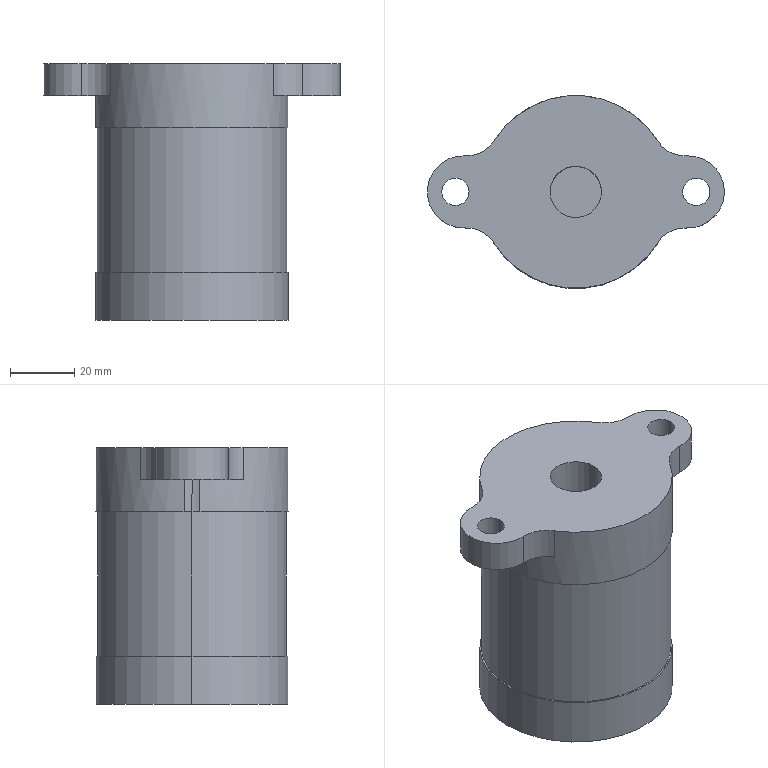Part | SolidWorks | features ICE 5, Cut 2, Extrusion 1, Fillet 1 | 1 solid | 33 faces | box 92.5 x 60 x 80 mm | volume 214232 mm3 | cylinder 23 | plane 10 | commonest cylinder face diameters 16 x6 8.5 x4 20 x4 60 x4 22.5 x3 59 x2
STEP:
#1=CARTESIAN_POINT('',(45.5,0.,-9.));
#2=VERTEX_POINT('',#1);
#3=CARTESIAN_POINT('',(29.5,0.,-9.));
#4=VERTEX_POINT('',#3);
#5=CARTESIAN_POINT('',(37.5,0.,-9.));
#6=DIRECTION('',(0.,0.,-1.));
#7=DIRECTION('',(-1.,0.,0.));
#8=AXIS2_PLACEMENT_3D('',#5,#6,#7);
#9=CIRCLE('',#8,8.);
#10=EDGE_CURVE('',#2,#4,#9,.T.);
#11=ORIENTED_EDGE('',*,*,#10,.F.);
#12=CARTESIAN_POINT('',(45.5,0.,-10.));
#13=VERTEX_POINT('',#12);
#14=CARTESIAN_POINT('',(45.5,0.,-9.));
#15=DIRECTION('',(0.,0.,-1.));
#16=VECTOR('',#15,1000.);
#17=LINE('',#14,#16);
#18=EDGE_CURVE('',#2,#13,#17,.T.);
#19=ORIENTED_EDGE('',*,*,#18,.T.);
#20=CARTESIAN_POINT('',(29.897,-2.488,-10.));
#21=VERTEX_POINT('',#20);
#22=CARTESIAN_POINT('',(37.5,0.,-10.));
#23=DIRECTION('',(0.,0.,-1.));
#24=DIRECTION('',(-1.,0.,0.));
#25=AXIS2_PLACEMENT_3D('',#22,#23,#24);
#26=CIRCLE('',#25,8.);
#27=EDGE_CURVE('',#13,#21,#26,.T.);
#28=ORIENTED_EDGE('',*,*,#27,.T.);
#29=CARTESIAN_POINT('',(29.897,-2.488,-20.));
#30=VERTEX_POINT('',#29);
#31=CARTESIAN_POINT('',(29.897,-2.488,-10.));
#32=DIRECTION('',(0.,0.,-1.));
#33=VECTOR('',#32,1000.);
#34=LINE('',#31,#33);
#35=EDGE_CURVE('',#21,#30,#34,.T.);
#36=ORIENTED_EDGE('',*,*,#35,.T.);
#37=CARTESIAN_POINT('',(29.5,0.,-20.));
#38=VERTEX_POINT('',#37);
#39=CARTESIAN_POINT('',(37.5,0.,-20.));
#40=DIRECTION('',(0.,0.,1.));
#41=DIRECTION('',(1.,0.,0.));
#42=AXIS2_PLACEMENT_3D('',#39,#40,#41);
#43=CIRCLE('',#42,8.);
#44=EDGE_CURVE('',#38,#30,#43,.T.);
#45=ORIENTED_EDGE('',*,*,#44,.F.);
#46=CARTESIAN_POINT('',(29.5,0.,-9.));
#47=DIRECTION('',(0.,0.,-1.));
#48=VECTOR('',#47,1000.);
#49=LINE('',#46,#48);
#50=EDGE_CURVE('',#4,#38,#49,.T.);
#51=ORIENTED_EDGE('',*,*,#50,.F.);
#52=EDGE_LOOP('',(#11,#19,#28,#36,#45,#51));
#53=FACE_OUTER_BOUND('',#52,.T.);
#54=CARTESIAN_POINT('',(37.5,0.,-9.));
#55=DIRECTION('',(0.,0.,-1.));
#56=DIRECTION('',(-1.,0.,0.));
#57=AXIS2_PLACEMENT_3D('',#54,#55,#56);
#58=CYLINDRICAL_SURFACE('',#57,8.);
#59=ADVANCED_FACE('',(#53),#58,.F.);
#60=CARTESIAN_POINT('',(-29.5,0.,-9.));
#61=VERTEX_POINT('',#60);
#62=CARTESIAN_POINT('',(-45.5,0.,-9.));
#63=VERTEX_POINT('',#62);
#64=CARTESIAN_POINT('',(-37.5,0.,-9.));
#65=DIRECTION('',(0.,0.,-1.));
#66=DIRECTION('',(-1.,0.,0.));
#67=AXIS2_PLACEMENT_3D('',#64,#65,#66);
#68=CIRCLE('',#67,8.);
#69=EDGE_CURVE('',#61,#63,#68,.T.);
#70=ORIENTED_EDGE('',*,*,#69,.F.);
#71=CARTESIAN_POINT('',(-29.5,0.,-20.));
#72=VERTEX_POINT('',#71);
#73=CARTESIAN_POINT('',(-29.5,0.,-9.));
#74=DIRECTION('',(0.,0.,-1.));
#75=VECTOR('',#74,1000.);
#76=LINE('',#73,#75);
#77=EDGE_CURVE('',#61,#72,#76,.T.);
#78=ORIENTED_EDGE('',*,*,#77,.T.);
#79=CARTESIAN_POINT('',(-29.897,-2.488,-20.));
#80=VERTEX_POINT('',#79);
#81=CARTESIAN_POINT('',(-37.5,0.,-20.));
#82=DIRECTION('',(0.,0.,1.));
#83=DIRECTION('',(1.,0.,0.));
#84=AXIS2_PLACEMENT_3D('',#81,#82,#83);
#85=CIRCLE('',#84,8.);
#86=EDGE_CURVE('',#80,#72,#85,.T.);
#87=ORIENTED_EDGE('',*,*,#86,.F.);
#88=CARTESIAN_POINT('',(-29.897,-2.488,-10.));
#89=VERTEX_POINT('',#88);
#90=CARTESIAN_POINT('',(-29.897,-2.488,-10.));
#91=DIRECTION('',(0.,0.,1.));
#92=VECTOR('',#91,1000.);
#93=LINE('',#90,#92);
#94=EDGE_CURVE('',#80,#89,#93,.T.);
#95=ORIENTED_EDGE('',*,*,#94,.T.);
#96=CARTESIAN_POINT('',(-45.5,0.,-10.));
#97=VERTEX_POINT('',#96);
#98=CARTESIAN_POINT('',(-37.5,0.,-10.));
#99=DIRECTION('',(0.,0.,-1.));
#100=DIRECTION('',(-1.,0.,0.));
#101=AXIS2_PLACEMENT_3D('',#98,#99,#100);
#102=CIRCLE('',#101,8.);
#103=EDGE_CURVE('',#89,#97,#102,.T.);
#104=ORIENTED_EDGE('',*,*,#103,.T.);
#105=CARTESIAN_POINT('',(-45.5,0.,-9.));
#106=DIRECTION('',(0.,0.,-1.));
#107=VECTOR('',#106,1000.);
#108=LINE('',#105,#107);
#109=EDGE_CURVE('',#63,#97,#108,.T.);
#110=ORIENTED_EDGE('',*,*,#109,.F.);
#111=EDGE_LOOP('',(#70,#78,#87,#95,#104,#110));
#112=FACE_OUTER_BOUND('',#111,.T.);
#113=CARTESIAN_POINT('',(-37.5,0.,-9.));
#114=DIRECTION('',(0.,0.,-1.));
#115=DIRECTION('',(-1.,0.,0.));
#116=AXIS2_PLACEMENT_3D('',#113,#114,#115);
#117=CYLINDRICAL_SURFACE('',#116,8.);
#118=ADVANCED_FACE('',(#112),#117,.F.);
#119=CARTESIAN_POINT('',(34.421,-11.235,-10.));
#120=VERTEX_POINT('',#119);
#121=CARTESIAN_POINT('',(46.25,0.,-10.));
#122=VERTEX_POINT('',#121);
#123=CARTESIAN_POINT('',(35.,0.,-10.));
#124=DIRECTION('',(0.,0.,1.));
#125=DIRECTION('',(1.,0.,0.));
#126=AXIS2_PLACEMENT_3D('',#123,#124,#125);
#127=CIRCLE('',#126,11.25);
#128=EDGE_CURVE('',#120,#122,#127,.T.);
#129=ORIENTED_EDGE('',*,*,#128,.T.);
#130=CARTESIAN_POINT('',(46.25,0.,0.));
#131=VERTEX_POINT('',#130);
#132=CARTESIAN_POINT('',(46.25,0.,-10.));
#133=DIRECTION('',(0.,0.,1.));
#134=VECTOR('',#133,1000.);
#135=LINE('',#132,#134);
#136=EDGE_CURVE('',#122,#131,#135,.T.);
#137=ORIENTED_EDGE('',*,*,#136,.T.);
#138=CARTESIAN_POINT('',(34.421,-11.235,0.));
#139=VERTEX_POINT('',#138);
#140=CARTESIAN_POINT('',(35.,0.,0.));
#141=DIRECTION('',(0.,0.,1.));
#142=DIRECTION('',(1.,0.,0.));
#143=AXIS2_PLACEMENT_3D('',#140,#141,#142);
#144=CIRCLE('',#143,11.25);
#145=EDGE_CURVE('',#139,#131,#144,.T.);
#146=ORIENTED_EDGE('',*,*,#145,.F.);
#147=CARTESIAN_POINT('',(34.421,-11.235,-10.));
#148=DIRECTION('',(0.,0.,-1.));
#149=VECTOR('',#148,1000.);
#150=LINE('',#147,#149);
#151=EDGE_CURVE('',#139,#120,#150,.T.);
#152=ORIENTED_EDGE('',*,*,#151,.T.);
#153=EDGE_LOOP('',(#129,#137,#146,#152));
#154=FACE_OUTER_BOUND('',#153,.T.);
#155=CARTESIAN_POINT('',(35.,0.,-10.));
#156=DIRECTION('',(0.,0.,1.));
#157=DIRECTION('',(1.,0.,0.));
#158=AXIS2_PLACEMENT_3D('',#155,#156,#157);
#159=CYLINDRICAL_SURFACE('',#158,11.25);
#160=ADVANCED_FACE('',(#154),#159,.T.);
#161=CARTESIAN_POINT('',(-8.,0.,-65.));
#162=VERTEX_POINT('',#161);
#163=CARTESIAN_POINT('',(8.,0.,-65.));
#164=VERTEX_POINT('',#163);
#165=CARTESIAN_POINT('',(0.,0.,-65.));
#166=DIRECTION('',(0.,0.,1.));
#167=DIRECTION('',(1.,0.,0.));
#168=AXIS2_PLACEMENT_3D('',#165,#166,#167);
#169=CIRCLE('',#168,8.);
#170=EDGE_CURVE('',#162,#164,#169,.T.);
#171=ORIENTED_EDGE('',*,*,#170,.F.);
#172=CARTESIAN_POINT('',(-8.,0.,0.));
#173=VERTEX_POINT('',#172);
#174=CARTESIAN_POINT('',(-8.,0.,-65.));
#175=DIRECTION('',(0.,0.,1.));
#176=VECTOR('',#175,1000.);
#177=LINE('',#174,#176);
#178=EDGE_CURVE('',#162,#173,#177,.T.);
#179=ORIENTED_EDGE('',*,*,#178,.T.);
#180=CARTESIAN_POINT('',(8.,0.,0.));
#181=VERTEX_POINT('',#180);
#182=CARTESIAN_POINT('',(0.,0.,0.));
#183=DIRECTION('',(0.,0.,1.));
#184=DIRECTION('',(1.,0.,0.));
#185=AXIS2_PLACEMENT_3D('',#182,#183,#184);
#186=CIRCLE('',#185,8.);
#187=EDGE_CURVE('',#173,#181,#186,.T.);
#188=ORIENTED_EDGE('',*,*,#187,.T.);
#189=CARTESIAN_POINT('',(8.,0.,-65.));
#190=DIRECTION('',(0.,0.,1.));
#191=VECTOR('',#190,1000.);
#192=LINE('',#189,#191);
#193=EDGE_CURVE('',#164,#181,#192,.T.);
#194=ORIENTED_EDGE('',*,*,#193,.F.);
#195=EDGE_LOOP('',(#171,#179,#188,#194));
#196=FACE_OUTER_BOUND('',#195,.T.);
#197=CARTESIAN_POINT('',(0.,0.,-65.));
#198=DIRECTION('',(0.,0.,1.));
#199=DIRECTION('',(1.,0.,0.));
#200=AXIS2_PLACEMENT_3D('',#197,#198,#199);
#201=CYLINDRICAL_SURFACE('',#200,8.);
#202=ADVANCED_FACE('',(#196),#201,.F.);
#203=CARTESIAN_POINT('',(-30.,0.,-80.));
#204=VERTEX_POINT('',#203);
#205=CARTESIAN_POINT('',(30.,0.,-80.));
#206=VERTEX_POINT('',#205);
#207=CARTESIAN_POINT('',(0.,0.,-80.));
#208=DIRECTION('',(0.,0.,-1.));
#209=DIRECTION('',(-1.,0.,0.));
#210=AXIS2_PLACEMENT_3D('',#207,#208,#209);
#211=CIRCLE('',#210,30.);
#212=EDGE_CURVE('',#204,#206,#211,.T.);
#213=ORIENTED_EDGE('',*,*,#212,.F.);
#214=CARTESIAN_POINT('',(-30.,0.,-65.));
#215=VERTEX_POINT('',#214);
#216=CARTESIAN_POINT('',(-30.,0.,-80.));
#217=DIRECTION('',(0.,0.,1.));
#218=VECTOR('',#217,1000.);
#219=LINE('',#216,#218);
#220=EDGE_CURVE('',#204,#215,#219,.T.);
#221=ORIENTED_EDGE('',*,*,#220,.T.);
#222=CARTESIAN_POINT('',(30.,0.,-65.));
#223=VERTEX_POINT('',#222);
#224=CARTESIAN_POINT('',(0.,0.,-65.));
#225=DIRECTION('',(0.,0.,-1.));
#226=DIRECTION('',(-1.,0.,0.));
#227=AXIS2_PLACEMENT_3D('',#224,#225,#226);
#228=CIRCLE('',#227,30.);
#229=EDGE_CURVE('',#215,#223,#228,.T.);
#230=ORIENTED_EDGE('',*,*,#229,.T.);
#231=CARTESIAN_POINT('',(30.,0.,-80.));
#232=DIRECTION('',(0.,0.,1.));
#233=VECTOR('',#232,1000.);
#234=LINE('',#231,#233);
#235=EDGE_CURVE('',#206,#223,#234,.T.);
#236=ORIENTED_EDGE('',*,*,#235,.F.);
#237=EDGE_LOOP('',(#213,#221,#230,#236));
#238=FACE_OUTER_BOUND('',#237,.T.);
#239=CARTESIAN_POINT('',(0.,0.,-80.));
#240=DIRECTION('',(0.,0.,1.));
#241=DIRECTION('',(1.,0.,0.));
#242=AXIS2_PLACEMENT_3D('',#239,#240,#241);
#243=CYLINDRICAL_SURFACE('',#242,30.);
#244=ADVANCED_FACE('',(#238),#243,.T.);
#245=CARTESIAN_POINT('',(-29.5,0.,-65.));
#246=VERTEX_POINT('',#245);
#247=CARTESIAN_POINT('',(29.5,0.,-65.));
#248=VERTEX_POINT('',#247);
#249=CARTESIAN_POINT('',(0.,0.,-65.));
#250=DIRECTION('',(0.,0.,-1.));
#251=DIRECTION('',(-1.,0.,0.));
#252=AXIS2_PLACEMENT_3D('',#249,#250,#251);
#253=CIRCLE('',#252,29.5);
#254=EDGE_CURVE('',#246,#248,#253,.T.);
#255=ORIENTED_EDGE('',*,*,#254,.F.);
#256=CARTESIAN_POINT('',(-29.5,0.,-65.));
#257=DIRECTION('',(0.,0.,1.));
#258=VECTOR('',#257,1000.);
#259=LINE('',#256,#258);
#260=EDGE_CURVE('',#246,#72,#259,.T.);
#261=ORIENTED_EDGE('',*,*,#260,.T.);
#262=CARTESIAN_POINT('',(0.,0.,-20.));
#263=DIRECTION('',(0.,0.,-1.));
#264=DIRECTION('',(1.,0.,0.));
#265=AXIS2_PLACEMENT_3D('',#262,#263,#264);
#266=CIRCLE('',#265,29.5);
#267=EDGE_CURVE('',#72,#38,#266,.T.);
#268=ORIENTED_EDGE('',*,*,#267,.T.);
#269=CARTESIAN_POINT('',(29.5,0.,-65.));
#270=DIRECTION('',(0.,0.,1.));
#271=VECTOR('',#270,1000.);
#272=LINE('',#269,#271);
#273=EDGE_CURVE('',#248,#38,#272,.T.);
#274=ORIENTED_EDGE('',*,*,#273,.F.);
#275=EDGE_LOOP('',(#255,#261,#268,#274));
#276=FACE_OUTER_BOUND('',#275,.T.);
#277=CARTESIAN_POINT('',(0.,0.,-65.));
#278=DIRECTION('',(0.,0.,1.));
#279=DIRECTION('',(1.,0.,0.));
#280=AXIS2_PLACEMENT_3D('',#277,#278,#279);
#281=CYLINDRICAL_SURFACE('',#280,29.5);
#282=ADVANCED_FACE('',(#276),#281,.T.);
#283=CARTESIAN_POINT('',(-33.25,0.,0.));
#284=VERTEX_POINT('',#283);
#285=CARTESIAN_POINT('',(-41.75,0.,0.));
#286=VERTEX_POINT('',#285);
#287=CARTESIAN_POINT('',(-37.5,0.,0.));
#288=DIRECTION('',(0.,0.,-1.));
#289=DIRECTION('',(-1.,0.,0.));
#290=AXIS2_PLACEMENT_3D('',#287,#288,#289);
#291=CIRCLE('',#290,4.25);
#292=EDGE_CURVE('',#284,#286,#291,.T.);
#293=ORIENTED_EDGE('',*,*,#292,.F.);
#294=CARTESIAN_POINT('',(-33.25,0.,-9.));
#295=VERTEX_POINT('',#294);
#296=CARTESIAN_POINT('',(-33.25,0.,0.));
#297=DIRECTION('',(0.,0.,-1.));
#298=VECTOR('',#297,1000.);
#299=LINE('',#296,#298);
#300=EDGE_CURVE('',#284,#295,#299,.T.);
#301=ORIENTED_EDGE('',*,*,#300,.T.);
#302=CARTESIAN_POINT('',(-41.75,0.,-9.));
#303=VERTEX_POINT('',#302);
#304=CARTESIAN_POINT('',(-37.5,0.,-9.));
#305=DIRECTION('',(0.,0.,1.));
#306=DIRECTION('',(-1.,0.,0.));
#307=AXIS2_PLACEMENT_3D('',#304,#305,#306);
#308=CIRCLE('',#307,4.25);
#309=EDGE_CURVE('',#303,#295,#308,.T.);
#310=ORIENTED_EDGE('',*,*,#309,.F.);
#311=CARTESIAN_POINT('',(-41.75,0.,0.));
#312=DIRECTION('',(0.,0.,-1.));
#313=VECTOR('',#312,1000.);
#314=LINE('',#311,#313);
#315=EDGE_CURVE('',#286,#303,#314,.T.);
#316=ORIENTED_EDGE('',*,*,#315,.F.);
#317=EDGE_LOOP('',(#293,#301,#310,#316));
#318=FACE_OUTER_BOUND('',#317,.T.);
#319=CARTESIAN_POINT('',(-37.5,0.,0.));
#320=DIRECTION('',(0.,0.,-1.));
#321=DIRECTION('',(-1.,0.,0.));
#322=AXIS2_PLACEMENT_3D('',#319,#320,#321);
#323=CYLINDRICAL_SURFACE('',#322,4.25);
#324=ADVANCED_FACE('',(#318),#323,.F.);
#325=CARTESIAN_POINT('',(41.75,0.,0.));
#326=VERTEX_POINT('',#325);
#327=CARTESIAN_POINT('',(33.25,0.,0.));
#328=VERTEX_POINT('',#327);
#329=CARTESIAN_POINT('',(37.5,0.,0.));
#330=DIRECTION('',(0.,0.,-1.));
#331=DIRECTION('',(-1.,0.,0.));
#332=AXIS2_PLACEMENT_3D('',#329,#330,#331);
#333=CIRCLE('',#332,4.25);
#334=EDGE_CURVE('',#326,#328,#333,.T.);
#335=ORIENTED_EDGE('',*,*,#334,.F.);
#336=CARTESIAN_POINT('',(41.75,0.,-9.));
#337=VERTEX_POINT('',#336);
#338=CARTESIAN_POINT('',(41.75,0.,0.));
#339=DIRECTION('',(0.,0.,-1.));
#340=VECTOR('',#339,1000.);
#341=LINE('',#338,#340);
#342=EDGE_CURVE('',#326,#337,#341,.T.);
#343=ORIENTED_EDGE('',*,*,#342,.T.);
#344=CARTESIAN_POINT('',(33.25,0.,-9.));
#345=VERTEX_POINT('',#344);
#346=CARTESIAN_POINT('',(37.5,0.,-9.));
#347=DIRECTION('',(0.,0.,1.));
#348=DIRECTION('',(-1.,0.,0.));
#349=AXIS2_PLACEMENT_3D('',#346,#347,#348);
#350=CIRCLE('',#349,4.25);
#351=EDGE_CURVE('',#345,#337,#350,.T.);
#352=ORIENTED_EDGE('',*,*,#351,.F.);
#353=CARTESIAN_POINT('',(33.25,0.,0.));
#354=DIRECTION('',(0.,0.,-1.));
#355=VECTOR('',#354,1000.);
#356=LINE('',#353,#355);
#357=EDGE_CURVE('',#328,#345,#356,.T.);
#358=ORIENTED_EDGE('',*,*,#357,.F.);
#359=EDGE_LOOP('',(#335,#343,#352,#358));
#360=FACE_OUTER_BOUND('',#359,.T.);
#361=CARTESIAN_POINT('',(37.5,0.,0.));
#362=DIRECTION('',(0.,0.,-1.));
#363=DIRECTION('',(-1.,0.,0.));
#364=AXIS2_PLACEMENT_3D('',#361,#362,#363);
#365=CYLINDRICAL_SURFACE('',#364,4.25);
#366=ADVANCED_FACE('',(#360),#365,.F.);
#367=ORIENTED_EDGE('',*,*,#44,.T.);
#368=CARTESIAN_POINT('',(0.,0.,-20.));
#369=DIRECTION('',(0.,0.,1.));
#370=DIRECTION('',(1.,0.,0.));
#371=AXIS2_PLACEMENT_3D('',#368,#369,#370);
#372=CIRCLE('',#371,30.);
#373=EDGE_CURVE('',#80,#30,#372,.T.);
#374=ORIENTED_EDGE('',*,*,#373,.F.);
#375=ORIENTED_EDGE('',*,*,#86,.T.);
#376=CARTESIAN_POINT('',(0.,0.,-20.));
#377=DIRECTION('',(0.,0.,-1.));
#378=DIRECTION('',(1.,0.,0.));
#379=AXIS2_PLACEMENT_3D('',#376,#377,#378);
#380=CIRCLE('',#379,29.5);
#381=EDGE_CURVE('',#38,#72,#380,.T.);
#382=ORIENTED_EDGE('',*,*,#381,.F.);
#383=EDGE_LOOP('',(#367,#374,#375,#382));
#384=FACE_OUTER_BOUND('',#383,.T.);
#385=CARTESIAN_POINT('',(0.,0.,-20.));
#386=DIRECTION('',(0.,0.,1.));
#387=DIRECTION('',(1.,0.,0.));
#388=AXIS2_PLACEMENT_3D('',#385,#386,#387);
#389=PLANE('',#388);
#390=ADVANCED_FACE('',(#384),#389,.F.);
#391=CARTESIAN_POINT('',(29.897,2.488,-20.));
#392=VERTEX_POINT('',#391);
#393=CARTESIAN_POINT('',(37.5,0.,-20.));
#394=DIRECTION('',(0.,0.,1.));
#395=DIRECTION('',(1.,0.,0.));
#396=AXIS2_PLACEMENT_3D('',#393,#394,#395);
#397=CIRCLE('',#396,8.);
#398=EDGE_CURVE('',#392,#38,#397,.T.);
#399=ORIENTED_EDGE('',*,*,#398,.T.);
#400=ORIENTED_EDGE('',*,*,#267,.F.);
#401=CARTESIAN_POINT('',(-29.897,2.488,-20.));
#402=VERTEX_POINT('',#401);
#403=CARTESIAN_POINT('',(-37.5,0.,-20.));
#404=DIRECTION('',(0.,0.,1.));
#405=DIRECTION('',(1.,0.,0.));
#406=AXIS2_PLACEMENT_3D('',#403,#404,#405);
#407=CIRCLE('',#406,8.);
#408=EDGE_CURVE('',#72,#402,#407,.T.);
#409=ORIENTED_EDGE('',*,*,#408,.T.);
#410=CARTESIAN_POINT('',(0.,0.,-20.));
#411=DIRECTION('',(0.,0.,1.));
#412=DIRECTION('',(1.,0.,0.));
#413=AXIS2_PLACEMENT_3D('',#410,#411,#412);
#414=CIRCLE('',#413,30.);
#415=EDGE_CURVE('',#392,#402,#414,.T.);
#416=ORIENTED_EDGE('',*,*,#415,.F.);
#417=EDGE_LOOP('',(#399,#400,#409,#416));
#418=FACE_OUTER_BOUND('',#417,.T.);
#419=CARTESIAN_POINT('',(0.,0.,-20.));
#420=DIRECTION('',(0.,0.,1.));
#421=DIRECTION('',(1.,0.,0.));
#422=AXIS2_PLACEMENT_3D('',#419,#420,#421);
#423=PLANE('',#422);
#424=ADVANCED_FACE('',(#418),#423,.F.);
#425=CARTESIAN_POINT('',(25.43,15.916,-10.));
#426=VERTEX_POINT('',#425);
#427=CARTESIAN_POINT('',(29.897,2.488,-10.));
#428=VERTEX_POINT('',#427);
#429=CARTESIAN_POINT('',(0.,0.,-10.));
#430=DIRECTION('',(0.,0.,-1.));
#431=DIRECTION('',(1.,0.,0.));
#432=AXIS2_PLACEMENT_3D('',#429,#430,#431);
#433=CIRCLE('',#432,30.);
#434=EDGE_CURVE('',#426,#428,#433,.T.);
#435=ORIENTED_EDGE('',*,*,#434,.T.);
#436=CARTESIAN_POINT('',(29.897,2.488,-10.));
#437=DIRECTION('',(0.,0.,1.));
#438=VECTOR('',#437,1000.);
#439=LINE('',#436,#438);
#440=EDGE_CURVE('',#392,#428,#439,.T.);
#441=ORIENTED_EDGE('',*,*,#440,.F.);
#442=ORIENTED_EDGE('',*,*,#415,.T.);
#443=CARTESIAN_POINT('',(-29.897,2.488,-10.));
#444=VERTEX_POINT('',#443);
#445=CARTESIAN_POINT('',(-29.897,2.488,-10.));
#446=DIRECTION('',(0.,0.,-1.));
#447=VECTOR('',#446,1000.);
#448=LINE('',#445,#447);
#449=EDGE_CURVE('',#444,#402,#448,.T.);
#450=ORIENTED_EDGE('',*,*,#449,.F.);
#451=CARTESIAN_POINT('',(-25.43,15.916,-10.));
#452=VERTEX_POINT('',#451);
#453=CARTESIAN_POINT('',(0.,0.,-10.));
#454=DIRECTION('',(0.,0.,-1.));
#455=DIRECTION('',(1.,0.,0.));
#456=AXIS2_PLACEMENT_3D('',#453,#454,#455);
#457=CIRCLE('',#456,30.);
#458=EDGE_CURVE('',#444,#452,#457,.T.);
#459=ORIENTED_EDGE('',*,*,#458,.T.);
#460=CARTESIAN_POINT('',(-25.43,15.916,0.));
#461=VERTEX_POINT('',#460);
#462=CARTESIAN_POINT('',(-25.43,15.916,-20.));
#463=DIRECTION('',(0.,0.,1.));
#464=VECTOR('',#463,1000.);
#465=LINE('',#462,#464);
#466=EDGE_CURVE('',#452,#461,#465,.T.);
#467=ORIENTED_EDGE('',*,*,#466,.T.);
#468=CARTESIAN_POINT('',(25.43,15.916,0.));
#469=VERTEX_POINT('',#468);
#470=CARTESIAN_POINT('',(0.,0.,0.));
#471=DIRECTION('',(0.,0.,1.));
#472=DIRECTION('',(1.,0.,0.));
#473=AXIS2_PLACEMENT_3D('',#470,#471,#472);
#474=CIRCLE('',#473,30.);
#475=EDGE_CURVE('',#469,#461,#474,.T.);
#476=ORIENTED_EDGE('',*,*,#475,.F.);
#477=CARTESIAN_POINT('',(25.43,15.916,-20.));
#478=DIRECTION('',(0.,0.,-1.));
#479=VECTOR('',#478,1000.);
#480=LINE('',#477,#479);
#481=EDGE_CURVE('',#469,#426,#480,.T.);
#482=ORIENTED_EDGE('',*,*,#481,.T.);
#483=EDGE_LOOP('',(#435,#441,#442,#450,#459,#467,#476,#482));
#484=FACE_OUTER_BOUND('',#483,.T.);
#485=CARTESIAN_POINT('',(0.,0.,-20.));
#486=DIRECTION('',(0.,0.,1.));
#487=DIRECTION('',(1.,0.,0.));
#488=AXIS2_PLACEMENT_3D('',#485,#486,#487);
#489=CYLINDRICAL_SURFACE('',#488,30.);
#490=ADVANCED_FACE('',(#484),#489,.T.);
#491=ORIENTED_EDGE('',*,*,#373,.T.);
#492=ORIENTED_EDGE('',*,*,#35,.F.);
#493=CARTESIAN_POINT('',(25.43,-15.916,-10.));
#494=VERTEX_POINT('',#493);
#495=CARTESIAN_POINT('',(0.,0.,-10.));
#496=DIRECTION('',(0.,0.,-1.));
#497=DIRECTION('',(1.,0.,0.));
#498=AXIS2_PLACEMENT_3D('',#495,#496,#497);
#499=CIRCLE('',#498,30.);
#500=EDGE_CURVE('',#21,#494,#499,.T.);
#501=ORIENTED_EDGE('',*,*,#500,.T.);
#502=CARTESIAN_POINT('',(25.43,-15.916,0.));
#503=VERTEX_POINT('',#502);
#504=CARTESIAN_POINT('',(25.43,-15.916,-20.));
#505=DIRECTION('',(0.,0.,1.));
#506=VECTOR('',#505,1000.);
#507=LINE('',#504,#506);
#508=EDGE_CURVE('',#494,#503,#507,.T.);
#509=ORIENTED_EDGE('',*,*,#508,.T.);
#510=CARTESIAN_POINT('',(-25.43,-15.916,0.));
#511=VERTEX_POINT('',#510);
#512=CARTESIAN_POINT('',(0.,0.,0.));
#513=DIRECTION('',(0.,0.,1.));
#514=DIRECTION('',(1.,0.,0.));
#515=AXIS2_PLACEMENT_3D('',#512,#513,#514);
#516=CIRCLE('',#515,30.);
#517=EDGE_CURVE('',#511,#503,#516,.T.);
#518=ORIENTED_EDGE('',*,*,#517,.F.);
#519=CARTESIAN_POINT('',(-25.43,-15.916,-10.));
#520=VERTEX_POINT('',#519);
#521=CARTESIAN_POINT('',(-25.43,-15.916,-20.));
#522=DIRECTION('',(0.,0.,-1.));
#523=VECTOR('',#522,1000.);
#524=LINE('',#521,#523);
#525=EDGE_CURVE('',#511,#520,#524,.T.);
#526=ORIENTED_EDGE('',*,*,#525,.T.);
#527=CARTESIAN_POINT('',(0.,0.,-10.));
#528=DIRECTION('',(0.,0.,-1.));
#529=DIRECTION('',(1.,0.,0.));
#530=AXIS2_PLACEMENT_3D('',#527,#528,#529);
#531=CIRCLE('',#530,30.);
#532=EDGE_CURVE('',#520,#89,#531,.T.);
#533=ORIENTED_EDGE('',*,*,#532,.T.);
#534=ORIENTED_EDGE('',*,*,#94,.F.);
#535=EDGE_LOOP('',(#491,#492,#501,#509,#518,#526,#533,#534));
#536=FACE_OUTER_BOUND('',#535,.T.);
#537=CARTESIAN_POINT('',(0.,0.,-20.));
#538=DIRECTION('',(0.,0.,1.));
#539=DIRECTION('',(1.,0.,0.));
#540=AXIS2_PLACEMENT_3D('',#537,#538,#539);
#541=CYLINDRICAL_SURFACE('',#540,30.);
#542=ADVANCED_FACE('',(#536),#541,.T.);
#543=ORIENTED_EDGE('',*,*,#342,.F.);
#544=CARTESIAN_POINT('',(37.5,0.,0.));
#545=DIRECTION('',(0.,0.,-1.));
#546=DIRECTION('',(-1.,0.,0.));
#547=AXIS2_PLACEMENT_3D('',#544,#545,#546);
#548=CIRCLE('',#547,4.25);
#549=EDGE_CURVE('',#328,#326,#548,.T.);
#550=ORIENTED_EDGE('',*,*,#549,.F.);
#551=ORIENTED_EDGE('',*,*,#357,.T.);
#552=CARTESIAN_POINT('',(37.5,0.,-9.));
#553=DIRECTION('',(0.,0.,1.));
#554=DIRECTION('',(-1.,0.,0.));
#555=AXIS2_PLACEMENT_3D('',#552,#553,#554);
#556=CIRCLE('',#555,4.25);
#557=EDGE_CURVE('',#337,#345,#556,.T.);
#558=ORIENTED_EDGE('',*,*,#557,.F.);
#559=EDGE_LOOP('',(#543,#550,#551,#558));
#560=FACE_OUTER_BOUND('',#559,.T.);
#561=CARTESIAN_POINT('',(37.5,0.,0.));
#562=DIRECTION('',(0.,0.,-1.));
#563=DIRECTION('',(-1.,0.,0.));
#564=AXIS2_PLACEMENT_3D('',#561,#562,#563);
#565=CYLINDRICAL_SURFACE('',#564,4.25);
#566=ADVANCED_FACE('',(#560),#565,.F.);
#567=ORIENTED_EDGE('',*,*,#300,.F.);
#568=CARTESIAN_POINT('',(-37.5,0.,0.));
#569=DIRECTION('',(0.,0.,-1.));
#570=DIRECTION('',(-1.,0.,0.));
#571=AXIS2_PLACEMENT_3D('',#568,#569,#570);
#572=CIRCLE('',#571,4.25);
#573=EDGE_CURVE('',#286,#284,#572,.T.);
#574=ORIENTED_EDGE('',*,*,#573,.F.);
#575=ORIENTED_EDGE('',*,*,#315,.T.);
#576=CARTESIAN_POINT('',(-37.5,0.,-9.));
#577=DIRECTION('',(0.,0.,1.));
#578=DIRECTION('',(-1.,0.,0.));
#579=AXIS2_PLACEMENT_3D('',#576,#577,#578);
#580=CIRCLE('',#579,4.25);
#581=EDGE_CURVE('',#295,#303,#580,.T.);
#582=ORIENTED_EDGE('',*,*,#581,.F.);
#583=EDGE_LOOP('',(#567,#574,#575,#582));
#584=FACE_OUTER_BOUND('',#583,.T.);
#585=CARTESIAN_POINT('',(-37.5,0.,0.));
#586=DIRECTION('',(0.,0.,-1.));
#587=DIRECTION('',(-1.,0.,0.));
#588=AXIS2_PLACEMENT_3D('',#585,#586,#587);
#589=CYLINDRICAL_SURFACE('',#588,4.25);
#590=ADVANCED_FACE('',(#584),#589,.F.);
#591=ORIENTED_EDGE('',*,*,#549,.T.);
#592=ORIENTED_EDGE('',*,*,#334,.T.);
#593=EDGE_LOOP('',(#591,#592));
#594=FACE_BOUND('',#593,.T.);
#595=ORIENTED_EDGE('',*,*,#573,.T.);
#596=ORIENTED_EDGE('',*,*,#292,.T.);
#597=EDGE_LOOP('',(#595,#596));
#598=FACE_BOUND('',#597,.T.);
#599=ORIENTED_EDGE('',*,*,#145,.T.);
#600=CARTESIAN_POINT('',(34.421,11.235,0.));
#601=VERTEX_POINT('',#600);
#602=CARTESIAN_POINT('',(35.,0.,0.));
#603=DIRECTION('',(0.,0.,1.));
#604=DIRECTION('',(1.,0.,0.));
#605=AXIS2_PLACEMENT_3D('',#602,#603,#604);
#606=CIRCLE('',#605,11.25);
#607=EDGE_CURVE('',#131,#601,#606,.T.);
#608=ORIENTED_EDGE('',*,*,#607,.T.);
#609=CARTESIAN_POINT('',(33.906,21.222,0.));
#610=DIRECTION('',(0.,0.,-1.));
#611=DIRECTION('',(1.,0.,0.));
#612=AXIS2_PLACEMENT_3D('',#609,#610,#611);
#613=CIRCLE('',#612,10.);
#614=EDGE_CURVE('',#601,#469,#613,.T.);
#615=ORIENTED_EDGE('',*,*,#614,.T.);
#616=ORIENTED_EDGE('',*,*,#475,.T.);
#617=CARTESIAN_POINT('',(-34.421,11.235,0.));
#618=VERTEX_POINT('',#617);
#619=CARTESIAN_POINT('',(-33.906,21.222,0.));
#620=DIRECTION('',(0.,0.,-1.));
#621=DIRECTION('',(1.,0.,0.));
#622=AXIS2_PLACEMENT_3D('',#619,#620,#621);
#623=CIRCLE('',#622,10.);
#624=EDGE_CURVE('',#461,#618,#623,.T.);
#625=ORIENTED_EDGE('',*,*,#624,.T.);
#626=CARTESIAN_POINT('',(-34.421,-11.235,0.));
#627=VERTEX_POINT('',#626);
#628=CARTESIAN_POINT('',(-35.,0.,0.));
#629=DIRECTION('',(0.,0.,1.));
#630=DIRECTION('',(1.,0.,0.));
#631=AXIS2_PLACEMENT_3D('',#628,#629,#630);
#632=CIRCLE('',#631,11.25);
#633=EDGE_CURVE('',#618,#627,#632,.T.);
#634=ORIENTED_EDGE('',*,*,#633,.T.);
#635=CARTESIAN_POINT('',(-33.906,-21.222,0.));
#636=DIRECTION('',(0.,0.,-1.));
#637=DIRECTION('',(1.,0.,0.));
#638=AXIS2_PLACEMENT_3D('',#635,#636,#637);
#639=CIRCLE('',#638,10.);
#640=EDGE_CURVE('',#627,#511,#639,.T.);
#641=ORIENTED_EDGE('',*,*,#640,.T.);
#642=ORIENTED_EDGE('',*,*,#517,.T.);
#643=CARTESIAN_POINT('',(33.906,-21.222,0.));
#644=DIRECTION('',(0.,0.,-1.));
#645=DIRECTION('',(1.,0.,0.));
#646=AXIS2_PLACEMENT_3D('',#643,#644,#645);
#647=CIRCLE('',#646,10.);
#648=EDGE_CURVE('',#503,#139,#647,.T.);
#649=ORIENTED_EDGE('',*,*,#648,.T.);
#650=EDGE_LOOP('',(#599,#608,#615,#616,#625,#634,#641,#642,#649));
#651=FACE_OUTER_BOUND('',#650,.T.);
#652=CARTESIAN_POINT('',(0.,0.,0.));
#653=DIRECTION('',(0.,0.,1.));
#654=DIRECTION('',(1.,0.,0.));
#655=AXIS2_PLACEMENT_3D('',#652,#653,#654);
#656=CIRCLE('',#655,8.);
#657=EDGE_CURVE('',#181,#173,#656,.T.);
#658=ORIENTED_EDGE('',*,*,#657,.F.);
#659=ORIENTED_EDGE('',*,*,#187,.F.);
#660=EDGE_LOOP('',(#658,#659));
#661=FACE_BOUND('',#660,.T.);
#662=CARTESIAN_POINT('',(0.,0.,0.));
#663=DIRECTION('',(0.,0.,1.));
#664=DIRECTION('',(1.,0.,0.));
#665=AXIS2_PLACEMENT_3D('',#662,#663,#664);
#666=PLANE('',#665);
#667=ADVANCED_FACE('',(#594,#598,#651,#661),#666,.T.);
#668=ORIENTED_EDGE('',*,*,#260,.F.);
#669=CARTESIAN_POINT('',(0.,0.,-65.));
#670=DIRECTION('',(0.,0.,-1.));
#671=DIRECTION('',(-1.,0.,0.));
#672=AXIS2_PLACEMENT_3D('',#669,#670,#671);
#673=CIRCLE('',#672,29.5);
#674=EDGE_CURVE('',#248,#246,#673,.T.);
#675=ORIENTED_EDGE('',*,*,#674,.F.);
#676=ORIENTED_EDGE('',*,*,#273,.T.);
#677=ORIENTED_EDGE('',*,*,#381,.T.);
#678=EDGE_LOOP('',(#668,#675,#676,#677));
#679=FACE_OUTER_BOUND('',#678,.T.);
#680=CARTESIAN_POINT('',(0.,0.,-65.));
#681=DIRECTION('',(0.,0.,1.));
#682=DIRECTION('',(1.,0.,0.));
#683=AXIS2_PLACEMENT_3D('',#680,#681,#682);
#684=CYLINDRICAL_SURFACE('',#683,29.5);
#685=ADVANCED_FACE('',(#679),#684,.T.);
#686=CARTESIAN_POINT('',(0.,0.,-65.));
#687=DIRECTION('',(0.,0.,-1.));
#688=DIRECTION('',(-1.,0.,0.));
#689=AXIS2_PLACEMENT_3D('',#686,#687,#688);
#690=CIRCLE('',#689,30.);
#691=EDGE_CURVE('',#223,#215,#690,.T.);
#692=ORIENTED_EDGE('',*,*,#691,.F.);
#693=ORIENTED_EDGE('',*,*,#229,.F.);
#694=EDGE_LOOP('',(#692,#693));
#695=FACE_OUTER_BOUND('',#694,.T.);
#696=ORIENTED_EDGE('',*,*,#674,.T.);
#697=ORIENTED_EDGE('',*,*,#254,.T.);
#698=EDGE_LOOP('',(#696,#697));
#699=FACE_BOUND('',#698,.T.);
#700=CARTESIAN_POINT('',(0.,0.,-65.));
#701=DIRECTION('',(0.,0.,-1.));
#702=DIRECTION('',(-1.,0.,0.));
#703=AXIS2_PLACEMENT_3D('',#700,#701,#702);
#704=PLANE('',#703);
#705=ADVANCED_FACE('',(#695,#699),#704,.F.);
#706=ORIENTED_EDGE('',*,*,#220,.F.);
#707=CARTESIAN_POINT('',(0.,0.,-80.));
#708=DIRECTION('',(0.,0.,-1.));
#709=DIRECTION('',(-1.,0.,0.));
#710=AXIS2_PLACEMENT_3D('',#707,#708,#709);
#711=CIRCLE('',#710,30.);
#712=EDGE_CURVE('',#206,#204,#711,.T.);
#713=ORIENTED_EDGE('',*,*,#712,.F.);
#714=ORIENTED_EDGE('',*,*,#235,.T.);
#715=ORIENTED_EDGE('',*,*,#691,.T.);
#716=EDGE_LOOP('',(#706,#713,#714,#715));
#717=FACE_OUTER_BOUND('',#716,.T.);
#718=CARTESIAN_POINT('',(0.,0.,-80.));
#719=DIRECTION('',(0.,0.,1.));
#720=DIRECTION('',(1.,0.,0.));
#721=AXIS2_PLACEMENT_3D('',#718,#719,#720);
#722=CYLINDRICAL_SURFACE('',#721,30.);
#723=ADVANCED_FACE('',(#717),#722,.T.);
#724=ORIENTED_EDGE('',*,*,#712,.T.);
#725=ORIENTED_EDGE('',*,*,#212,.T.);
#726=EDGE_LOOP('',(#724,#725));
#727=FACE_OUTER_BOUND('',#726,.T.);
#728=CARTESIAN_POINT('',(0.,0.,-80.));
#729=DIRECTION('',(0.,0.,-1.));
#730=DIRECTION('',(-1.,0.,0.));
#731=AXIS2_PLACEMENT_3D('',#728,#729,#730);
#732=PLANE('',#731);
#733=ADVANCED_FACE('',(#727),#732,.T.);
#734=ORIENTED_EDGE('',*,*,#178,.F.);
#735=CARTESIAN_POINT('',(0.,0.,-65.));
#736=DIRECTION('',(0.,0.,1.));
#737=DIRECTION('',(1.,0.,0.));
#738=AXIS2_PLACEMENT_3D('',#735,#736,#737);
#739=CIRCLE('',#738,8.);
#740=EDGE_CURVE('',#164,#162,#739,.T.);
#741=ORIENTED_EDGE('',*,*,#740,.F.);
#742=ORIENTED_EDGE('',*,*,#193,.T.);
#743=ORIENTED_EDGE('',*,*,#657,.T.);
#744=EDGE_LOOP('',(#734,#741,#742,#743));
#745=FACE_OUTER_BOUND('',#744,.T.);
#746=CARTESIAN_POINT('',(0.,0.,-65.));
#747=DIRECTION('',(0.,0.,1.));
#748=DIRECTION('',(1.,0.,0.));
#749=AXIS2_PLACEMENT_3D('',#746,#747,#748);
#750=CYLINDRICAL_SURFACE('',#749,8.);
#751=ADVANCED_FACE('',(#745),#750,.F.);
#752=ORIENTED_EDGE('',*,*,#740,.T.);
#753=ORIENTED_EDGE('',*,*,#170,.T.);
#754=EDGE_LOOP('',(#752,#753));
#755=FACE_OUTER_BOUND('',#754,.T.);
#756=CARTESIAN_POINT('',(0.,0.,-65.));
#757=DIRECTION('',(0.,0.,1.));
#758=DIRECTION('',(1.,0.,0.));
#759=AXIS2_PLACEMENT_3D('',#756,#757,#758);
#760=PLANE('',#759);
#761=ADVANCED_FACE('',(#755),#760,.T.);
#762=ORIENTED_EDGE('',*,*,#136,.F.);
#763=CARTESIAN_POINT('',(34.421,11.235,-10.));
#764=VERTEX_POINT('',#763);
#765=CARTESIAN_POINT('',(35.,0.,-10.));
#766=DIRECTION('',(0.,0.,1.));
#767=DIRECTION('',(1.,0.,0.));
#768=AXIS2_PLACEMENT_3D('',#765,#766,#767);
#769=CIRCLE('',#768,11.25);
#770=EDGE_CURVE('',#122,#764,#769,.T.);
#771=ORIENTED_EDGE('',*,*,#770,.T.);
#772=CARTESIAN_POINT('',(34.421,11.235,-10.));
#773=DIRECTION('',(0.,0.,1.));
#774=VECTOR('',#773,1000.);
#775=LINE('',#772,#774);
#776=EDGE_CURVE('',#764,#601,#775,.T.);
#777=ORIENTED_EDGE('',*,*,#776,.T.);
#778=ORIENTED_EDGE('',*,*,#607,.F.);
#779=EDGE_LOOP('',(#762,#771,#777,#778));
#780=FACE_OUTER_BOUND('',#779,.T.);
#781=CARTESIAN_POINT('',(35.,0.,-10.));
#782=DIRECTION('',(0.,0.,1.));
#783=DIRECTION('',(1.,0.,0.));
#784=AXIS2_PLACEMENT_3D('',#781,#782,#783);
#785=CYLINDRICAL_SURFACE('',#784,11.25);
#786=ADVANCED_FACE('',(#780),#785,.T.);
#787=ORIENTED_EDGE('',*,*,#500,.F.);
#788=ORIENTED_EDGE('',*,*,#27,.F.);
#789=CARTESIAN_POINT('',(37.5,0.,-10.));
#790=DIRECTION('',(0.,0.,-1.));
#791=DIRECTION('',(-1.,0.,0.));
#792=AXIS2_PLACEMENT_3D('',#789,#790,#791);
#793=CIRCLE('',#792,8.);
#794=EDGE_CURVE('',#428,#13,#793,.T.);
#795=ORIENTED_EDGE('',*,*,#794,.F.);
#796=ORIENTED_EDGE('',*,*,#434,.F.);
#797=CARTESIAN_POINT('',(33.906,21.222,-10.));
#798=DIRECTION('',(0.,0.,1.));
#799=DIRECTION('',(1.,0.,0.));
#800=AXIS2_PLACEMENT_3D('',#797,#798,#799);
#801=CIRCLE('',#800,10.);
#802=EDGE_CURVE('',#426,#764,#801,.T.);
#803=ORIENTED_EDGE('',*,*,#802,.T.);
#804=ORIENTED_EDGE('',*,*,#770,.F.);
#805=ORIENTED_EDGE('',*,*,#128,.F.);
#806=CARTESIAN_POINT('',(33.906,-21.222,-10.));
#807=DIRECTION('',(0.,0.,1.));
#808=DIRECTION('',(1.,0.,0.));
#809=AXIS2_PLACEMENT_3D('',#806,#807,#808);
#810=CIRCLE('',#809,10.);
#811=EDGE_CURVE('',#120,#494,#810,.T.);
#812=ORIENTED_EDGE('',*,*,#811,.T.);
#813=EDGE_LOOP('',(#787,#788,#795,#796,#803,#804,#805,#812));
#814=FACE_OUTER_BOUND('',#813,.T.);
#815=CARTESIAN_POINT('',(35.,0.,-10.));
#816=DIRECTION('',(0.,0.,1.));
#817=DIRECTION('',(1.,0.,0.));
#818=AXIS2_PLACEMENT_3D('',#815,#816,#817);
#819=PLANE('',#818);
#820=ADVANCED_FACE('',(#814),#819,.F.);
#821=CARTESIAN_POINT('',(-34.421,11.235,-10.));
#822=VERTEX_POINT('',#821);
#823=CARTESIAN_POINT('',(-34.421,-11.235,-10.));
#824=VERTEX_POINT('',#823);
#825=CARTESIAN_POINT('',(-35.,0.,-10.));
#826=DIRECTION('',(0.,0.,1.));
#827=DIRECTION('',(1.,0.,0.));
#828=AXIS2_PLACEMENT_3D('',#825,#826,#827);
#829=CIRCLE('',#828,11.25);
#830=EDGE_CURVE('',#822,#824,#829,.T.);
#831=ORIENTED_EDGE('',*,*,#830,.T.);
#832=CARTESIAN_POINT('',(-34.421,-11.235,-10.));
#833=DIRECTION('',(0.,0.,1.));
#834=VECTOR('',#833,1000.);
#835=LINE('',#832,#834);
#836=EDGE_CURVE('',#824,#627,#835,.T.);
#837=ORIENTED_EDGE('',*,*,#836,.T.);
#838=ORIENTED_EDGE('',*,*,#633,.F.);
#839=CARTESIAN_POINT('',(-34.421,11.235,-10.));
#840=DIRECTION('',(0.,0.,-1.));
#841=VECTOR('',#840,1000.);
#842=LINE('',#839,#841);
#843=EDGE_CURVE('',#618,#822,#842,.T.);
#844=ORIENTED_EDGE('',*,*,#843,.T.);
#845=EDGE_LOOP('',(#831,#837,#838,#844));
#846=FACE_OUTER_BOUND('',#845,.T.);
#847=CARTESIAN_POINT('',(-35.,0.,-10.));
#848=DIRECTION('',(0.,0.,1.));
#849=DIRECTION('',(1.,0.,0.));
#850=AXIS2_PLACEMENT_3D('',#847,#848,#849);
#851=CYLINDRICAL_SURFACE('',#850,11.25);
#852=ADVANCED_FACE('',(#846),#851,.T.);
#853=ORIENTED_EDGE('',*,*,#458,.F.);
#854=CARTESIAN_POINT('',(-37.5,0.,-10.));
#855=DIRECTION('',(0.,0.,-1.));
#856=DIRECTION('',(-1.,0.,0.));
#857=AXIS2_PLACEMENT_3D('',#854,#855,#856);
#858=CIRCLE('',#857,8.);
#859=EDGE_CURVE('',#97,#444,#858,.T.);
#860=ORIENTED_EDGE('',*,*,#859,.F.);
#861=ORIENTED_EDGE('',*,*,#103,.F.);
#862=ORIENTED_EDGE('',*,*,#532,.F.);
#863=CARTESIAN_POINT('',(-33.906,-21.222,-10.));
#864=DIRECTION('',(0.,0.,1.));
#865=DIRECTION('',(1.,0.,0.));
#866=AXIS2_PLACEMENT_3D('',#863,#864,#865);
#867=CIRCLE('',#866,10.);
#868=EDGE_CURVE('',#520,#824,#867,.T.);
#869=ORIENTED_EDGE('',*,*,#868,.T.);
#870=ORIENTED_EDGE('',*,*,#830,.F.);
#871=CARTESIAN_POINT('',(-33.906,21.222,-10.));
#872=DIRECTION('',(0.,0.,1.));
#873=DIRECTION('',(1.,0.,0.));
#874=AXIS2_PLACEMENT_3D('',#871,#872,#873);
#875=CIRCLE('',#874,10.);
#876=EDGE_CURVE('',#822,#452,#875,.T.);
#877=ORIENTED_EDGE('',*,*,#876,.T.);
#878=EDGE_LOOP('',(#853,#860,#861,#862,#869,#870,#877));
#879=FACE_OUTER_BOUND('',#878,.T.);
#880=CARTESIAN_POINT('',(-35.,0.,-10.));
#881=DIRECTION('',(0.,0.,1.));
#882=DIRECTION('',(1.,0.,0.));
#883=AXIS2_PLACEMENT_3D('',#880,#881,#882);
#884=PLANE('',#883);
#885=ADVANCED_FACE('',(#879),#884,.F.);
#886=ORIENTED_EDGE('',*,*,#648,.F.);
#887=ORIENTED_EDGE('',*,*,#508,.F.);
#888=ORIENTED_EDGE('',*,*,#811,.F.);
#889=ORIENTED_EDGE('',*,*,#151,.F.);
#890=EDGE_LOOP('',(#886,#887,#888,#889));
#891=FACE_OUTER_BOUND('',#890,.T.);
#892=CARTESIAN_POINT('',(33.906,-21.222,-20.));
#893=DIRECTION('',(0.,0.,1.));
#894=DIRECTION('',(1.,0.,0.));
#895=AXIS2_PLACEMENT_3D('',#892,#893,#894);
#896=CYLINDRICAL_SURFACE('',#895,10.);
#897=ADVANCED_FACE('',(#891),#896,.F.);
#898=ORIENTED_EDGE('',*,*,#868,.F.);
#899=ORIENTED_EDGE('',*,*,#525,.F.);
#900=ORIENTED_EDGE('',*,*,#640,.F.);
#901=ORIENTED_EDGE('',*,*,#836,.F.);
#902=EDGE_LOOP('',(#898,#899,#900,#901));
#903=FACE_OUTER_BOUND('',#902,.T.);
#904=CARTESIAN_POINT('',(-33.906,-21.222,-20.));
#905=DIRECTION('',(0.,0.,-1.));
#906=DIRECTION('',(-1.,0.,0.));
#907=AXIS2_PLACEMENT_3D('',#904,#905,#906);
#908=CYLINDRICAL_SURFACE('',#907,10.);
#909=ADVANCED_FACE('',(#903),#908,.F.);
#910=ORIENTED_EDGE('',*,*,#802,.F.);
#911=ORIENTED_EDGE('',*,*,#481,.F.);
#912=ORIENTED_EDGE('',*,*,#614,.F.);
#913=ORIENTED_EDGE('',*,*,#776,.F.);
#914=EDGE_LOOP('',(#910,#911,#912,#913));
#915=FACE_OUTER_BOUND('',#914,.T.);
#916=CARTESIAN_POINT('',(33.906,21.222,-20.));
#917=DIRECTION('',(0.,0.,-1.));
#918=DIRECTION('',(-1.,0.,0.));
#919=AXIS2_PLACEMENT_3D('',#916,#917,#918);
#920=CYLINDRICAL_SURFACE('',#919,10.);
#921=ADVANCED_FACE('',(#915),#920,.F.);
#922=ORIENTED_EDGE('',*,*,#624,.F.);
#923=ORIENTED_EDGE('',*,*,#466,.F.);
#924=ORIENTED_EDGE('',*,*,#876,.F.);
#925=ORIENTED_EDGE('',*,*,#843,.F.);
#926=EDGE_LOOP('',(#922,#923,#924,#925));
#927=FACE_OUTER_BOUND('',#926,.T.);
#928=CARTESIAN_POINT('',(-33.906,21.222,-20.));
#929=DIRECTION('',(0.,0.,1.));
#930=DIRECTION('',(1.,0.,0.));
#931=AXIS2_PLACEMENT_3D('',#928,#929,#930);
#932=CYLINDRICAL_SURFACE('',#931,10.);
#933=ADVANCED_FACE('',(#927),#932,.F.);
#934=CARTESIAN_POINT('',(-37.5,0.,-9.));
#935=DIRECTION('',(0.,0.,-1.));
#936=DIRECTION('',(-1.,0.,0.));
#937=AXIS2_PLACEMENT_3D('',#934,#935,#936);
#938=CIRCLE('',#937,8.);
#939=EDGE_CURVE('',#63,#61,#938,.T.);
#940=ORIENTED_EDGE('',*,*,#939,.T.);
#941=ORIENTED_EDGE('',*,*,#69,.T.);
#942=EDGE_LOOP('',(#940,#941));
#943=FACE_OUTER_BOUND('',#942,.T.);
#944=ORIENTED_EDGE('',*,*,#309,.T.);
#945=ORIENTED_EDGE('',*,*,#581,.T.);
#946=EDGE_LOOP('',(#944,#945));
#947=FACE_BOUND('',#946,.T.);
#948=CARTESIAN_POINT('',(-37.5,0.,-9.));
#949=DIRECTION('',(0.,0.,-1.));
#950=DIRECTION('',(-1.,0.,0.));
#951=AXIS2_PLACEMENT_3D('',#948,#949,#950);
#952=PLANE('',#951);
#953=ADVANCED_FACE('',(#943,#947),#952,.T.);
#954=ORIENTED_EDGE('',*,*,#77,.F.);
#955=ORIENTED_EDGE('',*,*,#939,.F.);
#956=ORIENTED_EDGE('',*,*,#109,.T.);
#957=ORIENTED_EDGE('',*,*,#859,.T.);
#958=ORIENTED_EDGE('',*,*,#449,.T.);
#959=ORIENTED_EDGE('',*,*,#408,.F.);
#960=EDGE_LOOP('',(#954,#955,#956,#957,#958,#959));
#961=FACE_OUTER_BOUND('',#960,.T.);
#962=CARTESIAN_POINT('',(-37.5,0.,-9.));
#963=DIRECTION('',(0.,0.,-1.));
#964=DIRECTION('',(-1.,0.,0.));
#965=AXIS2_PLACEMENT_3D('',#962,#963,#964);
#966=CYLINDRICAL_SURFACE('',#965,8.);
#967=ADVANCED_FACE('',(#961),#966,.F.);
#968=CARTESIAN_POINT('',(37.5,0.,-9.));
#969=DIRECTION('',(0.,0.,-1.));
#970=DIRECTION('',(-1.,0.,0.));
#971=AXIS2_PLACEMENT_3D('',#968,#969,#970);
#972=CIRCLE('',#971,8.);
#973=EDGE_CURVE('',#4,#2,#972,.T.);
#974=ORIENTED_EDGE('',*,*,#973,.T.);
#975=ORIENTED_EDGE('',*,*,#10,.T.);
#976=EDGE_LOOP('',(#974,#975));
#977=FACE_OUTER_BOUND('',#976,.T.);
#978=ORIENTED_EDGE('',*,*,#351,.T.);
#979=ORIENTED_EDGE('',*,*,#557,.T.);
#980=EDGE_LOOP('',(#978,#979));
#981=FACE_BOUND('',#980,.T.);
#982=CARTESIAN_POINT('',(37.5,0.,-9.));
#983=DIRECTION('',(0.,0.,-1.));
#984=DIRECTION('',(-1.,0.,0.));
#985=AXIS2_PLACEMENT_3D('',#982,#983,#984);
#986=PLANE('',#985);
#987=ADVANCED_FACE('',(#977,#981),#986,.T.);
#988=ORIENTED_EDGE('',*,*,#18,.F.);
#989=ORIENTED_EDGE('',*,*,#973,.F.);
#990=ORIENTED_EDGE('',*,*,#50,.T.);
#991=ORIENTED_EDGE('',*,*,#398,.F.);
#992=ORIENTED_EDGE('',*,*,#440,.T.);
#993=ORIENTED_EDGE('',*,*,#794,.T.);
#994=EDGE_LOOP('',(#988,#989,#990,#991,#992,#993));
#995=FACE_OUTER_BOUND('',#994,.T.);
#996=CARTESIAN_POINT('',(37.5,0.,-9.));
#997=DIRECTION('',(0.,0.,-1.));
#998=DIRECTION('',(-1.,0.,0.));
#999=AXIS2_PLACEMENT_3D('',#996,#997,#998);
#1000=CYLINDRICAL_SURFACE('',#999,8.);
#1001=ADVANCED_FACE('',(#995),#1000,.F.);
#1002=CLOSED_SHELL('',(#59,#118,#160,#202,#244,#282,#324,#366,#390,#424,#490,#542,#566,#590,#667,#685,#705,#723,#733,#751,#761,#786,#820,#852,#885,#897,#909,#921,#933,#953,#967,#987,#1001));
#1003=MANIFOLD_SOLID_BREP('',#1002);
#1004=CARTESIAN_POINT('',(0.,0.,0.));
#1005=DIRECTION('',(0.,0.,1.));
#1006=DIRECTION('',(1.,0.,0.));
#1007=AXIS2_PLACEMENT_3D('',#1004,#1005,#1006);
#1008=(LENGTH_UNIT()NAMED_UNIT(*)SI_UNIT(.MILLI.,.METRE.));
#1009=UNCERTAINTY_MEASURE_WITH_UNIT(LENGTH_MEASURE(0.00001),#1008,'','');
#1010=(NAMED_UNIT(*)PLANE_ANGLE_UNIT()SI_UNIT($,.RADIAN.));
#1011=(NAMED_UNIT(*)SI_UNIT($,.STERADIAN.)SOLID_ANGLE_UNIT());
#1012=(GEOMETRIC_REPRESENTATION_CONTEXT(3)GLOBAL_UNCERTAINTY_ASSIGNED_CONTEXT((#1009))GLOBAL_UNIT_ASSIGNED_CONTEXT((#1008,#1010,#1011))REPRESENTATION_CONTEXT('',''));
#1013=ADVANCED_BREP_SHAPE_REPRESENTATION('',(#1003,#1007),#1012);